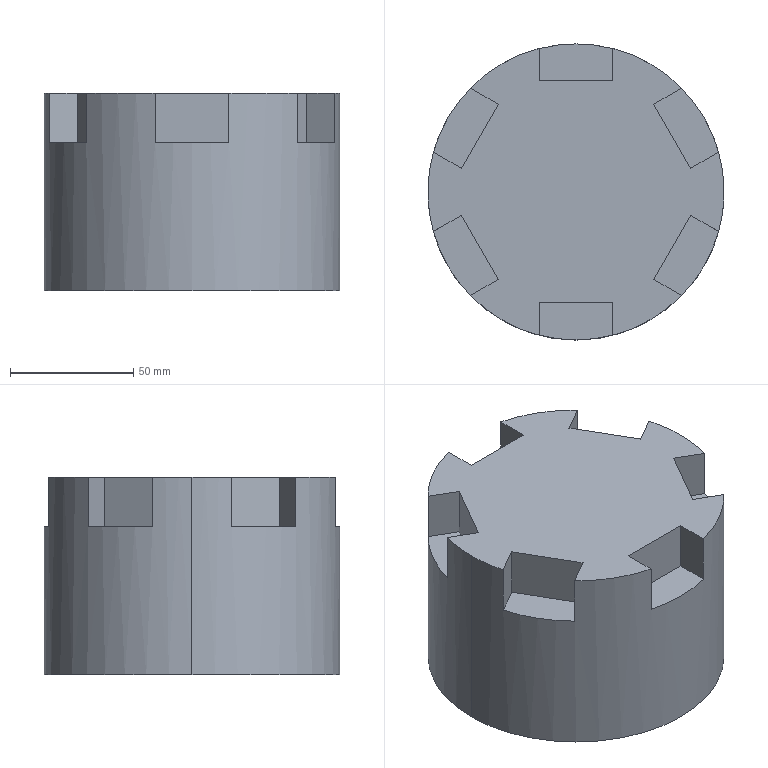Part | SolidWorks | features ICE 3, Extrusion 1 | 1 solid | 35 faces | box 120 x 120 x 80 mm | volume 586209 mm3 | plane 31 | cylinder 4 | commonest cylinder face diameters 75 x2 120 x2
STEP:
#1=CARTESIAN_POINT('',(60.,0.,80.));
#2=VERTEX_POINT('',#1);
#3=CARTESIAN_POINT('',(57.812,16.057,80.));
#4=VERTEX_POINT('',#3);
#5=CARTESIAN_POINT('',(0.,0.,80.));
#6=DIRECTION('',(0.,0.,1.));
#7=DIRECTION('',(1.,0.,0.));
#8=AXIS2_PLACEMENT_3D('',#5,#6,#7);
#9=CIRCLE('',#8,60.);
#10=EDGE_CURVE('',#2,#4,#9,.T.);
#11=ORIENTED_EDGE('',*,*,#10,.F.);
#12=CARTESIAN_POINT('',(60.,0.,0.));
#13=VERTEX_POINT('',#12);
#14=CARTESIAN_POINT('',(60.,0.,80.));
#15=DIRECTION('',(0.,0.,-1.));
#16=VECTOR('',#15,1000.);
#17=LINE('',#14,#16);
#18=EDGE_CURVE('',#2,#13,#17,.T.);
#19=ORIENTED_EDGE('',*,*,#18,.T.);
#20=CARTESIAN_POINT('',(-60.,0.,0.));
#21=VERTEX_POINT('',#20);
#22=CARTESIAN_POINT('',(0.,0.,0.));
#23=DIRECTION('',(0.,0.,1.));
#24=DIRECTION('',(1.,0.,0.));
#25=AXIS2_PLACEMENT_3D('',#22,#23,#24);
#26=CIRCLE('',#25,60.);
#27=EDGE_CURVE('',#13,#21,#26,.T.);
#28=ORIENTED_EDGE('',*,*,#27,.T.);
#29=CARTESIAN_POINT('',(-60.,0.,80.));
#30=VERTEX_POINT('',#29);
#31=CARTESIAN_POINT('',(-60.,0.,80.));
#32=DIRECTION('',(0.,0.,-1.));
#33=VECTOR('',#32,1000.);
#34=LINE('',#31,#33);
#35=EDGE_CURVE('',#30,#21,#34,.T.);
#36=ORIENTED_EDGE('',*,*,#35,.F.);
#37=CARTESIAN_POINT('',(-57.812,16.057,80.));
#38=VERTEX_POINT('',#37);
#39=CARTESIAN_POINT('',(0.,0.,80.));
#40=DIRECTION('',(0.,0.,1.));
#41=DIRECTION('',(1.,0.,0.));
#42=AXIS2_PLACEMENT_3D('',#39,#40,#41);
#43=CIRCLE('',#42,60.);
#44=EDGE_CURVE('',#38,#30,#43,.T.);
#45=ORIENTED_EDGE('',*,*,#44,.F.);
#46=CARTESIAN_POINT('',(-57.812,16.057,60.));
#47=VERTEX_POINT('',#46);
#48=CARTESIAN_POINT('',(-57.812,16.057,60.));
#49=DIRECTION('',(0.,0.,1.));
#50=VECTOR('',#49,1000.);
#51=LINE('',#48,#50);
#52=EDGE_CURVE('',#47,#38,#51,.T.);
#53=ORIENTED_EDGE('',*,*,#52,.F.);
#54=CARTESIAN_POINT('',(-42.812,42.038,60.));
#55=VERTEX_POINT('',#54);
#56=CARTESIAN_POINT('',(0.,0.,60.));
#57=DIRECTION('',(0.,0.,1.));
#58=DIRECTION('',(1.,0.,0.));
#59=AXIS2_PLACEMENT_3D('',#56,#57,#58);
#60=CIRCLE('',#59,60.);
#61=EDGE_CURVE('',#55,#47,#60,.T.);
#62=ORIENTED_EDGE('',*,*,#61,.F.);
#63=CARTESIAN_POINT('',(-42.812,42.038,80.));
#64=VERTEX_POINT('',#63);
#65=CARTESIAN_POINT('',(-42.812,42.038,60.));
#66=DIRECTION('',(0.,0.,1.));
#67=VECTOR('',#66,1000.);
#68=LINE('',#65,#67);
#69=EDGE_CURVE('',#55,#64,#68,.T.);
#70=ORIENTED_EDGE('',*,*,#69,.T.);
#71=CARTESIAN_POINT('',(-15.,58.095,80.));
#72=VERTEX_POINT('',#71);
#73=CARTESIAN_POINT('',(0.,0.,80.));
#74=DIRECTION('',(0.,0.,1.));
#75=DIRECTION('',(1.,0.,0.));
#76=AXIS2_PLACEMENT_3D('',#73,#74,#75);
#77=CIRCLE('',#76,60.);
#78=EDGE_CURVE('',#72,#64,#77,.T.);
#79=ORIENTED_EDGE('',*,*,#78,.F.);
#80=CARTESIAN_POINT('',(-15.,58.095,60.));
#81=VERTEX_POINT('',#80);
#82=CARTESIAN_POINT('',(-15.,58.095,60.));
#83=DIRECTION('',(0.,0.,1.));
#84=VECTOR('',#83,1000.);
#85=LINE('',#82,#84);
#86=EDGE_CURVE('',#81,#72,#85,.T.);
#87=ORIENTED_EDGE('',*,*,#86,.F.);
#88=CARTESIAN_POINT('',(15.,58.095,60.));
#89=VERTEX_POINT('',#88);
#90=CARTESIAN_POINT('',(0.,0.,60.));
#91=DIRECTION('',(0.,0.,1.));
#92=DIRECTION('',(1.,0.,0.));
#93=AXIS2_PLACEMENT_3D('',#90,#91,#92);
#94=CIRCLE('',#93,60.);
#95=EDGE_CURVE('',#89,#81,#94,.T.);
#96=ORIENTED_EDGE('',*,*,#95,.F.);
#97=CARTESIAN_POINT('',(15.,58.095,80.));
#98=VERTEX_POINT('',#97);
#99=CARTESIAN_POINT('',(15.,58.095,60.));
#100=DIRECTION('',(0.,0.,1.));
#101=VECTOR('',#100,1000.);
#102=LINE('',#99,#101);
#103=EDGE_CURVE('',#89,#98,#102,.T.);
#104=ORIENTED_EDGE('',*,*,#103,.T.);
#105=CARTESIAN_POINT('',(42.812,42.038,80.));
#106=VERTEX_POINT('',#105);
#107=CARTESIAN_POINT('',(0.,0.,80.));
#108=DIRECTION('',(0.,0.,1.));
#109=DIRECTION('',(1.,0.,0.));
#110=AXIS2_PLACEMENT_3D('',#107,#108,#109);
#111=CIRCLE('',#110,60.);
#112=EDGE_CURVE('',#106,#98,#111,.T.);
#113=ORIENTED_EDGE('',*,*,#112,.F.);
#114=CARTESIAN_POINT('',(42.812,42.038,60.));
#115=VERTEX_POINT('',#114);
#116=CARTESIAN_POINT('',(42.812,42.038,60.));
#117=DIRECTION('',(0.,0.,1.));
#118=VECTOR('',#117,1000.);
#119=LINE('',#116,#118);
#120=EDGE_CURVE('',#115,#106,#119,.T.);
#121=ORIENTED_EDGE('',*,*,#120,.F.);
#122=CARTESIAN_POINT('',(57.812,16.057,60.));
#123=VERTEX_POINT('',#122);
#124=CARTESIAN_POINT('',(0.,0.,60.));
#125=DIRECTION('',(0.,0.,1.));
#126=DIRECTION('',(1.,0.,0.));
#127=AXIS2_PLACEMENT_3D('',#124,#125,#126);
#128=CIRCLE('',#127,60.);
#129=EDGE_CURVE('',#123,#115,#128,.T.);
#130=ORIENTED_EDGE('',*,*,#129,.F.);
#131=CARTESIAN_POINT('',(57.812,16.057,60.));
#132=DIRECTION('',(0.,0.,1.));
#133=VECTOR('',#132,1000.);
#134=LINE('',#131,#133);
#135=EDGE_CURVE('',#123,#4,#134,.T.);
#136=ORIENTED_EDGE('',*,*,#135,.T.);
#137=EDGE_LOOP('',(#11,#19,#28,#36,#45,#53,#62,#70,#79,#87,#96,#104,#113,#121,#130,#136));
#138=FACE_OUTER_BOUND('',#137,.T.);
#139=CARTESIAN_POINT('',(0.,0.,80.));
#140=DIRECTION('',(0.,0.,-1.));
#141=DIRECTION('',(-1.,0.,0.));
#142=AXIS2_PLACEMENT_3D('',#139,#140,#141);
#143=CYLINDRICAL_SURFACE('',#142,60.);
#144=ADVANCED_FACE('',(#138),#143,.T.);
#145=CARTESIAN_POINT('',(-37.5,0.,60.));
#146=VERTEX_POINT('',#145);
#147=CARTESIAN_POINT('',(37.5,0.,60.));
#148=VERTEX_POINT('',#147);
#149=CARTESIAN_POINT('',(0.,0.,60.));
#150=DIRECTION('',(0.,0.,1.));
#151=DIRECTION('',(1.,0.,0.));
#152=AXIS2_PLACEMENT_3D('',#149,#150,#151);
#153=CIRCLE('',#152,37.5);
#154=EDGE_CURVE('',#146,#148,#153,.T.);
#155=ORIENTED_EDGE('',*,*,#154,.T.);
#156=CARTESIAN_POINT('',(37.5,0.,0.));
#157=VERTEX_POINT('',#156);
#158=CARTESIAN_POINT('',(37.5,0.,60.));
#159=DIRECTION('',(0.,0.,-1.));
#160=VECTOR('',#159,1000.);
#161=LINE('',#158,#160);
#162=EDGE_CURVE('',#148,#157,#161,.T.);
#163=ORIENTED_EDGE('',*,*,#162,.T.);
#164=CARTESIAN_POINT('',(-37.5,0.,0.));
#165=VERTEX_POINT('',#164);
#166=CARTESIAN_POINT('',(0.,0.,0.));
#167=DIRECTION('',(0.,0.,1.));
#168=DIRECTION('',(1.,0.,0.));
#169=AXIS2_PLACEMENT_3D('',#166,#167,#168);
#170=CIRCLE('',#169,37.5);
#171=EDGE_CURVE('',#165,#157,#170,.T.);
#172=ORIENTED_EDGE('',*,*,#171,.F.);
#173=CARTESIAN_POINT('',(-37.5,0.,60.));
#174=DIRECTION('',(0.,0.,-1.));
#175=VECTOR('',#174,1000.);
#176=LINE('',#173,#175);
#177=EDGE_CURVE('',#146,#165,#176,.T.);
#178=ORIENTED_EDGE('',*,*,#177,.F.);
#179=EDGE_LOOP('',(#155,#163,#172,#178));
#180=FACE_OUTER_BOUND('',#179,.T.);
#181=CARTESIAN_POINT('',(0.,0.,60.));
#182=DIRECTION('',(0.,0.,-1.));
#183=DIRECTION('',(-1.,0.,0.));
#184=AXIS2_PLACEMENT_3D('',#181,#182,#183);
#185=CYLINDRICAL_SURFACE('',#184,37.5);
#186=ADVANCED_FACE('',(#180),#185,.F.);
#187=CARTESIAN_POINT('',(0.,0.,0.));
#188=DIRECTION('',(0.,0.,1.));
#189=DIRECTION('',(1.,0.,0.));
#190=AXIS2_PLACEMENT_3D('',#187,#188,#189);
#191=CIRCLE('',#190,60.);
#192=EDGE_CURVE('',#21,#13,#191,.T.);
#193=ORIENTED_EDGE('',*,*,#192,.F.);
#194=ORIENTED_EDGE('',*,*,#27,.F.);
#195=EDGE_LOOP('',(#193,#194));
#196=FACE_OUTER_BOUND('',#195,.T.);
#197=CARTESIAN_POINT('',(-10.,40.,0.));
#198=VERTEX_POINT('',#197);
#199=CARTESIAN_POINT('',(-10.,36.142,0.));
#200=VERTEX_POINT('',#199);
#201=CARTESIAN_POINT('',(-10.,40.,0.));
#202=DIRECTION('',(0.,-1.,0.));
#203=VECTOR('',#202,1000.);
#204=LINE('',#201,#203);
#205=EDGE_CURVE('',#198,#200,#204,.T.);
#206=ORIENTED_EDGE('',*,*,#205,.T.);
#207=CARTESIAN_POINT('',(0.,0.,0.));
#208=DIRECTION('',(0.,0.,1.));
#209=DIRECTION('',(1.,0.,0.));
#210=AXIS2_PLACEMENT_3D('',#207,#208,#209);
#211=CIRCLE('',#210,37.5);
#212=EDGE_CURVE('',#200,#165,#211,.T.);
#213=ORIENTED_EDGE('',*,*,#212,.T.);
#214=ORIENTED_EDGE('',*,*,#171,.T.);
#215=CARTESIAN_POINT('',(10.,36.142,0.));
#216=VERTEX_POINT('',#215);
#217=CARTESIAN_POINT('',(0.,0.,0.));
#218=DIRECTION('',(0.,0.,1.));
#219=DIRECTION('',(1.,0.,0.));
#220=AXIS2_PLACEMENT_3D('',#217,#218,#219);
#221=CIRCLE('',#220,37.5);
#222=EDGE_CURVE('',#157,#216,#221,.T.);
#223=ORIENTED_EDGE('',*,*,#222,.T.);
#224=CARTESIAN_POINT('',(10.,40.,0.));
#225=VERTEX_POINT('',#224);
#226=CARTESIAN_POINT('',(10.,40.,0.));
#227=DIRECTION('',(0.,-1.,0.));
#228=VECTOR('',#227,1000.);
#229=LINE('',#226,#228);
#230=EDGE_CURVE('',#225,#216,#229,.T.);
#231=ORIENTED_EDGE('',*,*,#230,.F.);
#232=CARTESIAN_POINT('',(10.,40.,0.));
#233=DIRECTION('',(-1.,0.,0.));
#234=VECTOR('',#233,1000.);
#235=LINE('',#232,#234);
#236=EDGE_CURVE('',#225,#198,#235,.T.);
#237=ORIENTED_EDGE('',*,*,#236,.T.);
#238=EDGE_LOOP('',(#206,#213,#214,#223,#231,#237));
#239=FACE_BOUND('',#238,.T.);
#240=CARTESIAN_POINT('',(0.,0.,0.));
#241=DIRECTION('',(0.,0.,1.));
#242=DIRECTION('',(1.,0.,0.));
#243=AXIS2_PLACEMENT_3D('',#240,#241,#242);
#244=PLANE('',#243);
#245=ADVANCED_FACE('',(#196,#239),#244,.F.);
#246=ORIENTED_EDGE('',*,*,#162,.F.);
#247=CARTESIAN_POINT('',(0.,0.,60.));
#248=DIRECTION('',(0.,0.,1.));
#249=DIRECTION('',(1.,0.,0.));
#250=AXIS2_PLACEMENT_3D('',#247,#248,#249);
#251=CIRCLE('',#250,37.5);
#252=EDGE_CURVE('',#148,#146,#251,.T.);
#253=ORIENTED_EDGE('',*,*,#252,.T.);
#254=ORIENTED_EDGE('',*,*,#177,.T.);
#255=ORIENTED_EDGE('',*,*,#212,.F.);
#256=CARTESIAN_POINT('',(-10.,36.142,30.));
#257=VERTEX_POINT('',#256);
#258=CARTESIAN_POINT('',(-10.,36.142,60.));
#259=DIRECTION('',(0.,0.,1.));
#260=VECTOR('',#259,1000.);
#261=LINE('',#258,#260);
#262=EDGE_CURVE('',#200,#257,#261,.T.);
#263=ORIENTED_EDGE('',*,*,#262,.T.);
#264=CARTESIAN_POINT('',(10.,36.142,30.));
#265=VERTEX_POINT('',#264);
#266=CARTESIAN_POINT('',(0.,0.,30.));
#267=DIRECTION('',(0.,0.,1.));
#268=DIRECTION('',(1.,0.,0.));
#269=AXIS2_PLACEMENT_3D('',#266,#267,#268);
#270=CIRCLE('',#269,37.5);
#271=EDGE_CURVE('',#265,#257,#270,.T.);
#272=ORIENTED_EDGE('',*,*,#271,.F.);
#273=CARTESIAN_POINT('',(10.,36.142,60.));
#274=DIRECTION('',(0.,0.,1.));
#275=VECTOR('',#274,1000.);
#276=LINE('',#273,#275);
#277=EDGE_CURVE('',#216,#265,#276,.T.);
#278=ORIENTED_EDGE('',*,*,#277,.F.);
#279=ORIENTED_EDGE('',*,*,#222,.F.);
#280=EDGE_LOOP('',(#246,#253,#254,#255,#263,#272,#278,#279));
#281=FACE_OUTER_BOUND('',#280,.T.);
#282=CARTESIAN_POINT('',(0.,0.,60.));
#283=DIRECTION('',(0.,0.,-1.));
#284=DIRECTION('',(-1.,0.,0.));
#285=AXIS2_PLACEMENT_3D('',#282,#283,#284);
#286=CYLINDRICAL_SURFACE('',#285,37.5);
#287=ADVANCED_FACE('',(#281),#286,.F.);
#288=ORIENTED_EDGE('',*,*,#18,.F.);
#289=CARTESIAN_POINT('',(57.812,-16.057,80.));
#290=VERTEX_POINT('',#289);
#291=CARTESIAN_POINT('',(0.,0.,80.));
#292=DIRECTION('',(0.,0.,1.));
#293=DIRECTION('',(1.,0.,0.));
#294=AXIS2_PLACEMENT_3D('',#291,#292,#293);
#295=CIRCLE('',#294,60.);
#296=EDGE_CURVE('',#290,#2,#295,.T.);
#297=ORIENTED_EDGE('',*,*,#296,.F.);
#298=CARTESIAN_POINT('',(57.812,-16.057,60.));
#299=VERTEX_POINT('',#298);
#300=CARTESIAN_POINT('',(57.812,-16.057,60.));
#301=DIRECTION('',(0.,0.,1.));
#302=VECTOR('',#301,1000.);
#303=LINE('',#300,#302);
#304=EDGE_CURVE('',#299,#290,#303,.T.);
#305=ORIENTED_EDGE('',*,*,#304,.F.);
#306=CARTESIAN_POINT('',(42.812,-42.038,60.));
#307=VERTEX_POINT('',#306);
#308=CARTESIAN_POINT('',(0.,0.,60.));
#309=DIRECTION('',(0.,0.,1.));
#310=DIRECTION('',(1.,0.,0.));
#311=AXIS2_PLACEMENT_3D('',#308,#309,#310);
#312=CIRCLE('',#311,60.);
#313=EDGE_CURVE('',#307,#299,#312,.T.);
#314=ORIENTED_EDGE('',*,*,#313,.F.);
#315=CARTESIAN_POINT('',(42.812,-42.038,80.));
#316=VERTEX_POINT('',#315);
#317=CARTESIAN_POINT('',(42.812,-42.038,60.));
#318=DIRECTION('',(0.,0.,1.));
#319=VECTOR('',#318,1000.);
#320=LINE('',#317,#319);
#321=EDGE_CURVE('',#307,#316,#320,.T.);
#322=ORIENTED_EDGE('',*,*,#321,.T.);
#323=CARTESIAN_POINT('',(15.,-58.095,80.));
#324=VERTEX_POINT('',#323);
#325=CARTESIAN_POINT('',(0.,0.,80.));
#326=DIRECTION('',(0.,0.,1.));
#327=DIRECTION('',(1.,0.,0.));
#328=AXIS2_PLACEMENT_3D('',#325,#326,#327);
#329=CIRCLE('',#328,60.);
#330=EDGE_CURVE('',#324,#316,#329,.T.);
#331=ORIENTED_EDGE('',*,*,#330,.F.);
#332=CARTESIAN_POINT('',(15.,-58.095,60.));
#333=VERTEX_POINT('',#332);
#334=CARTESIAN_POINT('',(15.,-58.095,60.));
#335=DIRECTION('',(0.,0.,1.));
#336=VECTOR('',#335,1000.);
#337=LINE('',#334,#336);
#338=EDGE_CURVE('',#333,#324,#337,.T.);
#339=ORIENTED_EDGE('',*,*,#338,.F.);
#340=CARTESIAN_POINT('',(-15.,-58.095,60.));
#341=VERTEX_POINT('',#340);
#342=CARTESIAN_POINT('',(0.,0.,60.));
#343=DIRECTION('',(0.,0.,1.));
#344=DIRECTION('',(1.,0.,0.));
#345=AXIS2_PLACEMENT_3D('',#342,#343,#344);
#346=CIRCLE('',#345,60.);
#347=EDGE_CURVE('',#341,#333,#346,.T.);
#348=ORIENTED_EDGE('',*,*,#347,.F.);
#349=CARTESIAN_POINT('',(-15.,-58.095,80.));
#350=VERTEX_POINT('',#349);
#351=CARTESIAN_POINT('',(-15.,-58.095,60.));
#352=DIRECTION('',(0.,0.,1.));
#353=VECTOR('',#352,1000.);
#354=LINE('',#351,#353);
#355=EDGE_CURVE('',#341,#350,#354,.T.);
#356=ORIENTED_EDGE('',*,*,#355,.T.);
#357=CARTESIAN_POINT('',(-42.812,-42.038,80.));
#358=VERTEX_POINT('',#357);
#359=CARTESIAN_POINT('',(0.,0.,80.));
#360=DIRECTION('',(0.,0.,1.));
#361=DIRECTION('',(1.,0.,0.));
#362=AXIS2_PLACEMENT_3D('',#359,#360,#361);
#363=CIRCLE('',#362,60.);
#364=EDGE_CURVE('',#358,#350,#363,.T.);
#365=ORIENTED_EDGE('',*,*,#364,.F.);
#366=CARTESIAN_POINT('',(-42.812,-42.038,60.));
#367=VERTEX_POINT('',#366);
#368=CARTESIAN_POINT('',(-42.812,-42.038,60.));
#369=DIRECTION('',(0.,0.,1.));
#370=VECTOR('',#369,1000.);
#371=LINE('',#368,#370);
#372=EDGE_CURVE('',#367,#358,#371,.T.);
#373=ORIENTED_EDGE('',*,*,#372,.F.);
#374=CARTESIAN_POINT('',(-57.812,-16.057,60.));
#375=VERTEX_POINT('',#374);
#376=CARTESIAN_POINT('',(0.,0.,60.));
#377=DIRECTION('',(0.,0.,1.));
#378=DIRECTION('',(1.,0.,0.));
#379=AXIS2_PLACEMENT_3D('',#376,#377,#378);
#380=CIRCLE('',#379,60.);
#381=EDGE_CURVE('',#375,#367,#380,.T.);
#382=ORIENTED_EDGE('',*,*,#381,.F.);
#383=CARTESIAN_POINT('',(-57.812,-16.057,80.));
#384=VERTEX_POINT('',#383);
#385=CARTESIAN_POINT('',(-57.812,-16.057,60.));
#386=DIRECTION('',(0.,0.,1.));
#387=VECTOR('',#386,1000.);
#388=LINE('',#385,#387);
#389=EDGE_CURVE('',#375,#384,#388,.T.);
#390=ORIENTED_EDGE('',*,*,#389,.T.);
#391=CARTESIAN_POINT('',(0.,0.,80.));
#392=DIRECTION('',(0.,0.,1.));
#393=DIRECTION('',(1.,0.,0.));
#394=AXIS2_PLACEMENT_3D('',#391,#392,#393);
#395=CIRCLE('',#394,60.);
#396=EDGE_CURVE('',#30,#384,#395,.T.);
#397=ORIENTED_EDGE('',*,*,#396,.F.);
#398=ORIENTED_EDGE('',*,*,#35,.T.);
#399=ORIENTED_EDGE('',*,*,#192,.T.);
#400=EDGE_LOOP('',(#288,#297,#305,#314,#322,#331,#339,#348,#356,#365,#373,#382,#390,#397,#398,#399));
#401=FACE_OUTER_BOUND('',#400,.T.);
#402=CARTESIAN_POINT('',(0.,0.,80.));
#403=DIRECTION('',(0.,0.,-1.));
#404=DIRECTION('',(-1.,0.,0.));
#405=AXIS2_PLACEMENT_3D('',#402,#403,#404);
#406=CYLINDRICAL_SURFACE('',#405,60.);
#407=ADVANCED_FACE('',(#401),#406,.T.);
#408=CARTESIAN_POINT('',(15.,45.,80.));
#409=VERTEX_POINT('',#408);
#410=CARTESIAN_POINT('',(15.,58.095,80.));
#411=DIRECTION('',(0.,1.,0.));
#412=VECTOR('',#411,1000.);
#413=LINE('',#410,#412);
#414=EDGE_CURVE('',#409,#98,#413,.T.);
#415=ORIENTED_EDGE('',*,*,#414,.F.);
#416=CARTESIAN_POINT('',(-15.,45.,80.));
#417=VERTEX_POINT('',#416);
#418=CARTESIAN_POINT('',(-15.,45.,80.));
#419=DIRECTION('',(1.,0.,0.));
#420=VECTOR('',#419,1000.);
#421=LINE('',#418,#420);
#422=EDGE_CURVE('',#417,#409,#421,.T.);
#423=ORIENTED_EDGE('',*,*,#422,.F.);
#424=CARTESIAN_POINT('',(-15.,58.095,80.));
#425=DIRECTION('',(0.,-1.,0.));
#426=VECTOR('',#425,1000.);
#427=LINE('',#424,#426);
#428=EDGE_CURVE('',#72,#417,#427,.T.);
#429=ORIENTED_EDGE('',*,*,#428,.F.);
#430=ORIENTED_EDGE('',*,*,#78,.T.);
#431=CARTESIAN_POINT('',(-31.471,35.49,80.));
#432=VERTEX_POINT('',#431);
#433=CARTESIAN_POINT('',(-42.812,42.038,80.));
#434=DIRECTION('',(-0.866,0.5,0.));
#435=VECTOR('',#434,1000.);
#436=LINE('',#433,#435);
#437=EDGE_CURVE('',#432,#64,#436,.T.);
#438=ORIENTED_EDGE('',*,*,#437,.F.);
#439=CARTESIAN_POINT('',(-46.471,9.51,80.));
#440=VERTEX_POINT('',#439);
#441=CARTESIAN_POINT('',(-46.471,9.51,80.));
#442=DIRECTION('',(0.5,0.866,0.));
#443=VECTOR('',#442,1000.);
#444=LINE('',#441,#443);
#445=EDGE_CURVE('',#440,#432,#444,.T.);
#446=ORIENTED_EDGE('',*,*,#445,.F.);
#447=CARTESIAN_POINT('',(-57.812,16.057,80.));
#448=DIRECTION('',(0.866,-0.5,0.));
#449=VECTOR('',#448,1000.);
#450=LINE('',#447,#449);
#451=EDGE_CURVE('',#38,#440,#450,.T.);
#452=ORIENTED_EDGE('',*,*,#451,.F.);
#453=ORIENTED_EDGE('',*,*,#44,.T.);
#454=ORIENTED_EDGE('',*,*,#396,.T.);
#455=CARTESIAN_POINT('',(-46.471,-9.51,80.));
#456=VERTEX_POINT('',#455);
#457=CARTESIAN_POINT('',(-57.812,-16.057,80.));
#458=DIRECTION('',(-0.866,-0.5,0.));
#459=VECTOR('',#458,1000.);
#460=LINE('',#457,#459);
#461=EDGE_CURVE('',#456,#384,#460,.T.);
#462=ORIENTED_EDGE('',*,*,#461,.F.);
#463=CARTESIAN_POINT('',(-31.471,-35.49,80.));
#464=VERTEX_POINT('',#463);
#465=CARTESIAN_POINT('',(-31.471,-35.49,80.));
#466=DIRECTION('',(-0.5,0.866,0.));
#467=VECTOR('',#466,1000.);
#468=LINE('',#465,#467);
#469=EDGE_CURVE('',#464,#456,#468,.T.);
#470=ORIENTED_EDGE('',*,*,#469,.F.);
#471=CARTESIAN_POINT('',(-42.812,-42.038,80.));
#472=DIRECTION('',(0.866,0.5,0.));
#473=VECTOR('',#472,1000.);
#474=LINE('',#471,#473);
#475=EDGE_CURVE('',#358,#464,#474,.T.);
#476=ORIENTED_EDGE('',*,*,#475,.F.);
#477=ORIENTED_EDGE('',*,*,#364,.T.);
#478=CARTESIAN_POINT('',(-15.,-45.,80.));
#479=VERTEX_POINT('',#478);
#480=CARTESIAN_POINT('',(-15.,-58.095,80.));
#481=DIRECTION('',(0.,-1.,0.));
#482=VECTOR('',#481,1000.);
#483=LINE('',#480,#482);
#484=EDGE_CURVE('',#479,#350,#483,.T.);
#485=ORIENTED_EDGE('',*,*,#484,.F.);
#486=CARTESIAN_POINT('',(15.,-45.,80.));
#487=VERTEX_POINT('',#486);
#488=CARTESIAN_POINT('',(15.,-45.,80.));
#489=DIRECTION('',(-1.,0.,0.));
#490=VECTOR('',#489,1000.);
#491=LINE('',#488,#490);
#492=EDGE_CURVE('',#487,#479,#491,.T.);
#493=ORIENTED_EDGE('',*,*,#492,.F.);
#494=CARTESIAN_POINT('',(15.,-58.095,80.));
#495=DIRECTION('',(0.,1.,0.));
#496=VECTOR('',#495,1000.);
#497=LINE('',#494,#496);
#498=EDGE_CURVE('',#324,#487,#497,.T.);
#499=ORIENTED_EDGE('',*,*,#498,.F.);
#500=ORIENTED_EDGE('',*,*,#330,.T.);
#501=CARTESIAN_POINT('',(31.471,-35.49,80.));
#502=VERTEX_POINT('',#501);
#503=CARTESIAN_POINT('',(42.812,-42.038,80.));
#504=DIRECTION('',(0.866,-0.5,0.));
#505=VECTOR('',#504,1000.);
#506=LINE('',#503,#505);
#507=EDGE_CURVE('',#502,#316,#506,.T.);
#508=ORIENTED_EDGE('',*,*,#507,.F.);
#509=CARTESIAN_POINT('',(46.471,-9.51,80.));
#510=VERTEX_POINT('',#509);
#511=CARTESIAN_POINT('',(46.471,-9.51,80.));
#512=DIRECTION('',(-0.5,-0.866,0.));
#513=VECTOR('',#512,1000.);
#514=LINE('',#511,#513);
#515=EDGE_CURVE('',#510,#502,#514,.T.);
#516=ORIENTED_EDGE('',*,*,#515,.F.);
#517=CARTESIAN_POINT('',(57.812,-16.057,80.));
#518=DIRECTION('',(-0.866,0.5,0.));
#519=VECTOR('',#518,1000.);
#520=LINE('',#517,#519);
#521=EDGE_CURVE('',#290,#510,#520,.T.);
#522=ORIENTED_EDGE('',*,*,#521,.F.);
#523=ORIENTED_EDGE('',*,*,#296,.T.);
#524=ORIENTED_EDGE('',*,*,#10,.T.);
#525=CARTESIAN_POINT('',(46.471,9.51,80.));
#526=VERTEX_POINT('',#525);
#527=CARTESIAN_POINT('',(57.812,16.057,80.));
#528=DIRECTION('',(0.866,0.5,0.));
#529=VECTOR('',#528,1000.);
#530=LINE('',#527,#529);
#531=EDGE_CURVE('',#526,#4,#530,.T.);
#532=ORIENTED_EDGE('',*,*,#531,.F.);
#533=CARTESIAN_POINT('',(31.471,35.49,80.));
#534=VERTEX_POINT('',#533);
#535=CARTESIAN_POINT('',(31.471,35.49,80.));
#536=DIRECTION('',(0.5,-0.866,0.));
#537=VECTOR('',#536,1000.);
#538=LINE('',#535,#537);
#539=EDGE_CURVE('',#534,#526,#538,.T.);
#540=ORIENTED_EDGE('',*,*,#539,.F.);
#541=CARTESIAN_POINT('',(42.812,42.038,80.));
#542=DIRECTION('',(-0.866,-0.5,0.));
#543=VECTOR('',#542,1000.);
#544=LINE('',#541,#543);
#545=EDGE_CURVE('',#106,#534,#544,.T.);
#546=ORIENTED_EDGE('',*,*,#545,.F.);
#547=ORIENTED_EDGE('',*,*,#112,.T.);
#548=EDGE_LOOP('',(#415,#423,#429,#430,#438,#446,#452,#453,#454,#462,#470,#476,#477,#485,#493,#499,#500,#508,#516,#522,#523,#524,#532,#540,#546,#547));
#549=FACE_OUTER_BOUND('',#548,.T.);
#550=CARTESIAN_POINT('',(0.,0.,80.));
#551=DIRECTION('',(0.,0.,1.));
#552=DIRECTION('',(1.,0.,0.));
#553=AXIS2_PLACEMENT_3D('',#550,#551,#552);
#554=PLANE('',#553);
#555=ADVANCED_FACE('',(#549),#554,.T.);
#556=ORIENTED_EDGE('',*,*,#154,.F.);
#557=ORIENTED_EDGE('',*,*,#252,.F.);
#558=EDGE_LOOP('',(#556,#557));
#559=FACE_OUTER_BOUND('',#558,.T.);
#560=CARTESIAN_POINT('',(0.,0.,60.));
#561=DIRECTION('',(0.,0.,1.));
#562=DIRECTION('',(1.,0.,0.));
#563=AXIS2_PLACEMENT_3D('',#560,#561,#562);
#564=PLANE('',#563);
#565=ADVANCED_FACE('',(#559),#564,.F.);
#566=ORIENTED_EDGE('',*,*,#539,.T.);
#567=CARTESIAN_POINT('',(46.471,9.51,60.));
#568=VERTEX_POINT('',#567);
#569=CARTESIAN_POINT('',(46.471,9.51,60.));
#570=DIRECTION('',(0.,0.,1.));
#571=VECTOR('',#570,1000.);
#572=LINE('',#569,#571);
#573=EDGE_CURVE('',#568,#526,#572,.T.);
#574=ORIENTED_EDGE('',*,*,#573,.F.);
#575=CARTESIAN_POINT('',(31.471,35.49,60.));
#576=VERTEX_POINT('',#575);
#577=CARTESIAN_POINT('',(31.471,35.49,60.));
#578=DIRECTION('',(0.5,-0.866,0.));
#579=VECTOR('',#578,1000.);
#580=LINE('',#577,#579);
#581=EDGE_CURVE('',#576,#568,#580,.T.);
#582=ORIENTED_EDGE('',*,*,#581,.F.);
#583=CARTESIAN_POINT('',(31.471,35.49,60.));
#584=DIRECTION('',(0.,0.,1.));
#585=VECTOR('',#584,1000.);
#586=LINE('',#583,#585);
#587=EDGE_CURVE('',#576,#534,#586,.T.);
#588=ORIENTED_EDGE('',*,*,#587,.T.);
#589=EDGE_LOOP('',(#566,#574,#582,#588));
#590=FACE_OUTER_BOUND('',#589,.T.);
#591=CARTESIAN_POINT('',(31.471,35.49,60.));
#592=DIRECTION('',(-0.866,-0.5,0.));
#593=DIRECTION('',(0.5,-0.866,0.));
#594=AXIS2_PLACEMENT_3D('',#591,#592,#593);
#595=PLANE('',#594);
#596=ADVANCED_FACE('',(#590),#595,.F.);
#597=ORIENTED_EDGE('',*,*,#545,.T.);
#598=ORIENTED_EDGE('',*,*,#587,.F.);
#599=CARTESIAN_POINT('',(42.812,42.038,60.));
#600=DIRECTION('',(-0.866,-0.5,0.));
#601=VECTOR('',#600,1000.);
#602=LINE('',#599,#601);
#603=EDGE_CURVE('',#115,#576,#602,.T.);
#604=ORIENTED_EDGE('',*,*,#603,.F.);
#605=ORIENTED_EDGE('',*,*,#120,.T.);
#606=EDGE_LOOP('',(#597,#598,#604,#605));
#607=FACE_OUTER_BOUND('',#606,.T.);
#608=CARTESIAN_POINT('',(42.812,42.038,60.));
#609=DIRECTION('',(-0.5,0.866,0.));
#610=DIRECTION('',(-0.866,-0.5,0.));
#611=AXIS2_PLACEMENT_3D('',#608,#609,#610);
#612=PLANE('',#611);
#613=ADVANCED_FACE('',(#607),#612,.F.);
#614=ORIENTED_EDGE('',*,*,#531,.T.);
#615=ORIENTED_EDGE('',*,*,#135,.F.);
#616=CARTESIAN_POINT('',(57.812,16.057,60.));
#617=DIRECTION('',(0.866,0.5,0.));
#618=VECTOR('',#617,1000.);
#619=LINE('',#616,#618);
#620=EDGE_CURVE('',#568,#123,#619,.T.);
#621=ORIENTED_EDGE('',*,*,#620,.F.);
#622=ORIENTED_EDGE('',*,*,#573,.T.);
#623=EDGE_LOOP('',(#614,#615,#621,#622));
#624=FACE_OUTER_BOUND('',#623,.T.);
#625=CARTESIAN_POINT('',(57.812,16.057,60.));
#626=DIRECTION('',(0.5,-0.866,0.));
#627=DIRECTION('',(0.866,0.5,0.));
#628=AXIS2_PLACEMENT_3D('',#625,#626,#627);
#629=PLANE('',#628);
#630=ADVANCED_FACE('',(#624),#629,.F.);
#631=ORIENTED_EDGE('',*,*,#581,.T.);
#632=ORIENTED_EDGE('',*,*,#620,.T.);
#633=ORIENTED_EDGE('',*,*,#129,.T.);
#634=ORIENTED_EDGE('',*,*,#603,.T.);
#635=EDGE_LOOP('',(#631,#632,#633,#634));
#636=FACE_OUTER_BOUND('',#635,.T.);
#637=CARTESIAN_POINT('',(0.,0.,60.));
#638=DIRECTION('',(0.,0.,1.));
#639=DIRECTION('',(1.,0.,0.));
#640=AXIS2_PLACEMENT_3D('',#637,#638,#639);
#641=PLANE('',#640);
#642=ADVANCED_FACE('',(#636),#641,.T.);
#643=ORIENTED_EDGE('',*,*,#515,.T.);
#644=CARTESIAN_POINT('',(31.471,-35.49,60.));
#645=VERTEX_POINT('',#644);
#646=CARTESIAN_POINT('',(31.471,-35.49,60.));
#647=DIRECTION('',(0.,0.,1.));
#648=VECTOR('',#647,1000.);
#649=LINE('',#646,#648);
#650=EDGE_CURVE('',#645,#502,#649,.T.);
#651=ORIENTED_EDGE('',*,*,#650,.F.);
#652=CARTESIAN_POINT('',(46.471,-9.51,60.));
#653=VERTEX_POINT('',#652);
#654=CARTESIAN_POINT('',(46.471,-9.51,60.));
#655=DIRECTION('',(-0.5,-0.866,0.));
#656=VECTOR('',#655,1000.);
#657=LINE('',#654,#656);
#658=EDGE_CURVE('',#653,#645,#657,.T.);
#659=ORIENTED_EDGE('',*,*,#658,.F.);
#660=CARTESIAN_POINT('',(46.471,-9.51,60.));
#661=DIRECTION('',(0.,0.,1.));
#662=VECTOR('',#661,1000.);
#663=LINE('',#660,#662);
#664=EDGE_CURVE('',#653,#510,#663,.T.);
#665=ORIENTED_EDGE('',*,*,#664,.T.);
#666=EDGE_LOOP('',(#643,#651,#659,#665));
#667=FACE_OUTER_BOUND('',#666,.T.);
#668=CARTESIAN_POINT('',(46.471,-9.51,60.));
#669=DIRECTION('',(-0.866,0.5,0.));
#670=DIRECTION('',(-0.5,-0.866,0.));
#671=AXIS2_PLACEMENT_3D('',#668,#669,#670);
#672=PLANE('',#671);
#673=ADVANCED_FACE('',(#667),#672,.F.);
#674=ORIENTED_EDGE('',*,*,#521,.T.);
#675=ORIENTED_EDGE('',*,*,#664,.F.);
#676=CARTESIAN_POINT('',(57.812,-16.057,60.));
#677=DIRECTION('',(-0.866,0.5,0.));
#678=VECTOR('',#677,1000.);
#679=LINE('',#676,#678);
#680=EDGE_CURVE('',#299,#653,#679,.T.);
#681=ORIENTED_EDGE('',*,*,#680,.F.);
#682=ORIENTED_EDGE('',*,*,#304,.T.);
#683=EDGE_LOOP('',(#674,#675,#681,#682));
#684=FACE_OUTER_BOUND('',#683,.T.);
#685=CARTESIAN_POINT('',(57.812,-16.057,60.));
#686=DIRECTION('',(0.5,0.866,0.));
#687=DIRECTION('',(-0.866,0.5,0.));
#688=AXIS2_PLACEMENT_3D('',#685,#686,#687);
#689=PLANE('',#688);
#690=ADVANCED_FACE('',(#684),#689,.F.);
#691=ORIENTED_EDGE('',*,*,#507,.T.);
#692=ORIENTED_EDGE('',*,*,#321,.F.);
#693=CARTESIAN_POINT('',(42.812,-42.038,60.));
#694=DIRECTION('',(0.866,-0.5,0.));
#695=VECTOR('',#694,1000.);
#696=LINE('',#693,#695);
#697=EDGE_CURVE('',#645,#307,#696,.T.);
#698=ORIENTED_EDGE('',*,*,#697,.F.);
#699=ORIENTED_EDGE('',*,*,#650,.T.);
#700=EDGE_LOOP('',(#691,#692,#698,#699));
#701=FACE_OUTER_BOUND('',#700,.T.);
#702=CARTESIAN_POINT('',(42.812,-42.038,60.));
#703=DIRECTION('',(-0.5,-0.866,0.));
#704=DIRECTION('',(0.866,-0.5,0.));
#705=AXIS2_PLACEMENT_3D('',#702,#703,#704);
#706=PLANE('',#705);
#707=ADVANCED_FACE('',(#701),#706,.F.);
#708=ORIENTED_EDGE('',*,*,#658,.T.);
#709=ORIENTED_EDGE('',*,*,#697,.T.);
#710=ORIENTED_EDGE('',*,*,#313,.T.);
#711=ORIENTED_EDGE('',*,*,#680,.T.);
#712=EDGE_LOOP('',(#708,#709,#710,#711));
#713=FACE_OUTER_BOUND('',#712,.T.);
#714=CARTESIAN_POINT('',(0.,0.,60.));
#715=DIRECTION('',(0.,0.,1.));
#716=DIRECTION('',(1.,0.,0.));
#717=AXIS2_PLACEMENT_3D('',#714,#715,#716);
#718=PLANE('',#717);
#719=ADVANCED_FACE('',(#713),#718,.T.);
#720=ORIENTED_EDGE('',*,*,#492,.T.);
#721=CARTESIAN_POINT('',(-15.,-45.,60.));
#722=VERTEX_POINT('',#721);
#723=CARTESIAN_POINT('',(-15.,-45.,60.));
#724=DIRECTION('',(0.,0.,1.));
#725=VECTOR('',#724,1000.);
#726=LINE('',#723,#725);
#727=EDGE_CURVE('',#722,#479,#726,.T.);
#728=ORIENTED_EDGE('',*,*,#727,.F.);
#729=CARTESIAN_POINT('',(15.,-45.,60.));
#730=VERTEX_POINT('',#729);
#731=CARTESIAN_POINT('',(15.,-45.,60.));
#732=DIRECTION('',(-1.,0.,0.));
#733=VECTOR('',#732,1000.);
#734=LINE('',#731,#733);
#735=EDGE_CURVE('',#730,#722,#734,.T.);
#736=ORIENTED_EDGE('',*,*,#735,.F.);
#737=CARTESIAN_POINT('',(15.,-45.,60.));
#738=DIRECTION('',(0.,0.,1.));
#739=VECTOR('',#738,1000.);
#740=LINE('',#737,#739);
#741=EDGE_CURVE('',#730,#487,#740,.T.);
#742=ORIENTED_EDGE('',*,*,#741,.T.);
#743=EDGE_LOOP('',(#720,#728,#736,#742));
#744=FACE_OUTER_BOUND('',#743,.T.);
#745=CARTESIAN_POINT('',(15.,-45.,60.));
#746=DIRECTION('',(0.,1.,0.));
#747=DIRECTION('',(-1.,0.,0.));
#748=AXIS2_PLACEMENT_3D('',#745,#746,#747);
#749=PLANE('',#748);
#750=ADVANCED_FACE('',(#744),#749,.F.);
#751=ORIENTED_EDGE('',*,*,#498,.T.);
#752=ORIENTED_EDGE('',*,*,#741,.F.);
#753=CARTESIAN_POINT('',(15.,-58.095,60.));
#754=DIRECTION('',(0.,1.,0.));
#755=VECTOR('',#754,1000.);
#756=LINE('',#753,#755);
#757=EDGE_CURVE('',#333,#730,#756,.T.);
#758=ORIENTED_EDGE('',*,*,#757,.F.);
#759=ORIENTED_EDGE('',*,*,#338,.T.);
#760=EDGE_LOOP('',(#751,#752,#758,#759));
#761=FACE_OUTER_BOUND('',#760,.T.);
#762=CARTESIAN_POINT('',(15.,-58.095,60.));
#763=DIRECTION('',(1.,0.,0.));
#764=DIRECTION('',(0.,1.,0.));
#765=AXIS2_PLACEMENT_3D('',#762,#763,#764);
#766=PLANE('',#765);
#767=ADVANCED_FACE('',(#761),#766,.F.);
#768=ORIENTED_EDGE('',*,*,#484,.T.);
#769=ORIENTED_EDGE('',*,*,#355,.F.);
#770=CARTESIAN_POINT('',(-15.,-58.095,60.));
#771=DIRECTION('',(0.,-1.,0.));
#772=VECTOR('',#771,1000.);
#773=LINE('',#770,#772);
#774=EDGE_CURVE('',#722,#341,#773,.T.);
#775=ORIENTED_EDGE('',*,*,#774,.F.);
#776=ORIENTED_EDGE('',*,*,#727,.T.);
#777=EDGE_LOOP('',(#768,#769,#775,#776));
#778=FACE_OUTER_BOUND('',#777,.T.);
#779=CARTESIAN_POINT('',(-15.,-58.095,60.));
#780=DIRECTION('',(-1.,0.,0.));
#781=DIRECTION('',(0.,-1.,0.));
#782=AXIS2_PLACEMENT_3D('',#779,#780,#781);
#783=PLANE('',#782);
#784=ADVANCED_FACE('',(#778),#783,.F.);
#785=ORIENTED_EDGE('',*,*,#735,.T.);
#786=ORIENTED_EDGE('',*,*,#774,.T.);
#787=ORIENTED_EDGE('',*,*,#347,.T.);
#788=ORIENTED_EDGE('',*,*,#757,.T.);
#789=EDGE_LOOP('',(#785,#786,#787,#788));
#790=FACE_OUTER_BOUND('',#789,.T.);
#791=CARTESIAN_POINT('',(0.,0.,60.));
#792=DIRECTION('',(0.,0.,1.));
#793=DIRECTION('',(1.,0.,0.));
#794=AXIS2_PLACEMENT_3D('',#791,#792,#793);
#795=PLANE('',#794);
#796=ADVANCED_FACE('',(#790),#795,.T.);
#797=ORIENTED_EDGE('',*,*,#469,.T.);
#798=CARTESIAN_POINT('',(-46.471,-9.51,60.));
#799=VERTEX_POINT('',#798);
#800=CARTESIAN_POINT('',(-46.471,-9.51,60.));
#801=DIRECTION('',(0.,0.,1.));
#802=VECTOR('',#801,1000.);
#803=LINE('',#800,#802);
#804=EDGE_CURVE('',#799,#456,#803,.T.);
#805=ORIENTED_EDGE('',*,*,#804,.F.);
#806=CARTESIAN_POINT('',(-31.471,-35.49,60.));
#807=VERTEX_POINT('',#806);
#808=CARTESIAN_POINT('',(-31.471,-35.49,60.));
#809=DIRECTION('',(-0.5,0.866,0.));
#810=VECTOR('',#809,1000.);
#811=LINE('',#808,#810);
#812=EDGE_CURVE('',#807,#799,#811,.T.);
#813=ORIENTED_EDGE('',*,*,#812,.F.);
#814=CARTESIAN_POINT('',(-31.471,-35.49,60.));
#815=DIRECTION('',(0.,0.,1.));
#816=VECTOR('',#815,1000.);
#817=LINE('',#814,#816);
#818=EDGE_CURVE('',#807,#464,#817,.T.);
#819=ORIENTED_EDGE('',*,*,#818,.T.);
#820=EDGE_LOOP('',(#797,#805,#813,#819));
#821=FACE_OUTER_BOUND('',#820,.T.);
#822=CARTESIAN_POINT('',(-31.471,-35.49,60.));
#823=DIRECTION('',(0.866,0.5,0.));
#824=DIRECTION('',(-0.5,0.866,0.));
#825=AXIS2_PLACEMENT_3D('',#822,#823,#824);
#826=PLANE('',#825);
#827=ADVANCED_FACE('',(#821),#826,.F.);
#828=ORIENTED_EDGE('',*,*,#475,.T.);
#829=ORIENTED_EDGE('',*,*,#818,.F.);
#830=CARTESIAN_POINT('',(-42.812,-42.038,60.));
#831=DIRECTION('',(0.866,0.5,0.));
#832=VECTOR('',#831,1000.);
#833=LINE('',#830,#832);
#834=EDGE_CURVE('',#367,#807,#833,.T.);
#835=ORIENTED_EDGE('',*,*,#834,.F.);
#836=ORIENTED_EDGE('',*,*,#372,.T.);
#837=EDGE_LOOP('',(#828,#829,#835,#836));
#838=FACE_OUTER_BOUND('',#837,.T.);
#839=CARTESIAN_POINT('',(-42.812,-42.038,60.));
#840=DIRECTION('',(0.5,-0.866,0.));
#841=DIRECTION('',(0.866,0.5,0.));
#842=AXIS2_PLACEMENT_3D('',#839,#840,#841);
#843=PLANE('',#842);
#844=ADVANCED_FACE('',(#838),#843,.F.);
#845=ORIENTED_EDGE('',*,*,#461,.T.);
#846=ORIENTED_EDGE('',*,*,#389,.F.);
#847=CARTESIAN_POINT('',(-57.812,-16.057,60.));
#848=DIRECTION('',(-0.866,-0.5,0.));
#849=VECTOR('',#848,1000.);
#850=LINE('',#847,#849);
#851=EDGE_CURVE('',#799,#375,#850,.T.);
#852=ORIENTED_EDGE('',*,*,#851,.F.);
#853=ORIENTED_EDGE('',*,*,#804,.T.);
#854=EDGE_LOOP('',(#845,#846,#852,#853));
#855=FACE_OUTER_BOUND('',#854,.T.);
#856=CARTESIAN_POINT('',(-57.812,-16.057,60.));
#857=DIRECTION('',(-0.5,0.866,0.));
#858=DIRECTION('',(-0.866,-0.5,0.));
#859=AXIS2_PLACEMENT_3D('',#856,#857,#858);
#860=PLANE('',#859);
#861=ADVANCED_FACE('',(#855),#860,.F.);
#862=ORIENTED_EDGE('',*,*,#812,.T.);
#863=ORIENTED_EDGE('',*,*,#851,.T.);
#864=ORIENTED_EDGE('',*,*,#381,.T.);
#865=ORIENTED_EDGE('',*,*,#834,.T.);
#866=EDGE_LOOP('',(#862,#863,#864,#865));
#867=FACE_OUTER_BOUND('',#866,.T.);
#868=CARTESIAN_POINT('',(0.,0.,60.));
#869=DIRECTION('',(0.,0.,1.));
#870=DIRECTION('',(1.,0.,0.));
#871=AXIS2_PLACEMENT_3D('',#868,#869,#870);
#872=PLANE('',#871);
#873=ADVANCED_FACE('',(#867),#872,.T.);
#874=ORIENTED_EDGE('',*,*,#445,.T.);
#875=CARTESIAN_POINT('',(-31.471,35.49,60.));
#876=VERTEX_POINT('',#875);
#877=CARTESIAN_POINT('',(-31.471,35.49,60.));
#878=DIRECTION('',(0.,0.,1.));
#879=VECTOR('',#878,1000.);
#880=LINE('',#877,#879);
#881=EDGE_CURVE('',#876,#432,#880,.T.);
#882=ORIENTED_EDGE('',*,*,#881,.F.);
#883=CARTESIAN_POINT('',(-46.471,9.51,60.));
#884=VERTEX_POINT('',#883);
#885=CARTESIAN_POINT('',(-46.471,9.51,60.));
#886=DIRECTION('',(0.5,0.866,0.));
#887=VECTOR('',#886,1000.);
#888=LINE('',#885,#887);
#889=EDGE_CURVE('',#884,#876,#888,.T.);
#890=ORIENTED_EDGE('',*,*,#889,.F.);
#891=CARTESIAN_POINT('',(-46.471,9.51,60.));
#892=DIRECTION('',(0.,0.,1.));
#893=VECTOR('',#892,1000.);
#894=LINE('',#891,#893);
#895=EDGE_CURVE('',#884,#440,#894,.T.);
#896=ORIENTED_EDGE('',*,*,#895,.T.);
#897=EDGE_LOOP('',(#874,#882,#890,#896));
#898=FACE_OUTER_BOUND('',#897,.T.);
#899=CARTESIAN_POINT('',(-46.471,9.51,60.));
#900=DIRECTION('',(0.866,-0.5,0.));
#901=DIRECTION('',(0.5,0.866,0.));
#902=AXIS2_PLACEMENT_3D('',#899,#900,#901);
#903=PLANE('',#902);
#904=ADVANCED_FACE('',(#898),#903,.F.);
#905=ORIENTED_EDGE('',*,*,#451,.T.);
#906=ORIENTED_EDGE('',*,*,#895,.F.);
#907=CARTESIAN_POINT('',(-57.812,16.057,60.));
#908=DIRECTION('',(0.866,-0.5,0.));
#909=VECTOR('',#908,1000.);
#910=LINE('',#907,#909);
#911=EDGE_CURVE('',#47,#884,#910,.T.);
#912=ORIENTED_EDGE('',*,*,#911,.F.);
#913=ORIENTED_EDGE('',*,*,#52,.T.);
#914=EDGE_LOOP('',(#905,#906,#912,#913));
#915=FACE_OUTER_BOUND('',#914,.T.);
#916=CARTESIAN_POINT('',(-57.812,16.057,60.));
#917=DIRECTION('',(-0.5,-0.866,0.));
#918=DIRECTION('',(0.866,-0.5,0.));
#919=AXIS2_PLACEMENT_3D('',#916,#917,#918);
#920=PLANE('',#919);
#921=ADVANCED_FACE('',(#915),#920,.F.);
#922=ORIENTED_EDGE('',*,*,#437,.T.);
#923=ORIENTED_EDGE('',*,*,#69,.F.);
#924=CARTESIAN_POINT('',(-42.812,42.038,60.));
#925=DIRECTION('',(-0.866,0.5,0.));
#926=VECTOR('',#925,1000.);
#927=LINE('',#924,#926);
#928=EDGE_CURVE('',#876,#55,#927,.T.);
#929=ORIENTED_EDGE('',*,*,#928,.F.);
#930=ORIENTED_EDGE('',*,*,#881,.T.);
#931=EDGE_LOOP('',(#922,#923,#929,#930));
#932=FACE_OUTER_BOUND('',#931,.T.);
#933=CARTESIAN_POINT('',(-42.812,42.038,60.));
#934=DIRECTION('',(0.5,0.866,0.));
#935=DIRECTION('',(-0.866,0.5,0.));
#936=AXIS2_PLACEMENT_3D('',#933,#934,#935);
#937=PLANE('',#936);
#938=ADVANCED_FACE('',(#932),#937,.F.);
#939=ORIENTED_EDGE('',*,*,#889,.T.);
#940=ORIENTED_EDGE('',*,*,#928,.T.);
#941=ORIENTED_EDGE('',*,*,#61,.T.);
#942=ORIENTED_EDGE('',*,*,#911,.T.);
#943=EDGE_LOOP('',(#939,#940,#941,#942));
#944=FACE_OUTER_BOUND('',#943,.T.);
#945=CARTESIAN_POINT('',(0.,0.,60.));
#946=DIRECTION('',(0.,0.,1.));
#947=DIRECTION('',(1.,0.,0.));
#948=AXIS2_PLACEMENT_3D('',#945,#946,#947);
#949=PLANE('',#948);
#950=ADVANCED_FACE('',(#944),#949,.T.);
#951=ORIENTED_EDGE('',*,*,#414,.T.);
#952=ORIENTED_EDGE('',*,*,#103,.F.);
#953=CARTESIAN_POINT('',(15.,45.,60.));
#954=VERTEX_POINT('',#953);
#955=CARTESIAN_POINT('',(15.,58.095,60.));
#956=DIRECTION('',(0.,1.,0.));
#957=VECTOR('',#956,1000.);
#958=LINE('',#955,#957);
#959=EDGE_CURVE('',#954,#89,#958,.T.);
#960=ORIENTED_EDGE('',*,*,#959,.F.);
#961=CARTESIAN_POINT('',(15.,45.,60.));
#962=DIRECTION('',(0.,0.,1.));
#963=VECTOR('',#962,1000.);
#964=LINE('',#961,#963);
#965=EDGE_CURVE('',#954,#409,#964,.T.);
#966=ORIENTED_EDGE('',*,*,#965,.T.);
#967=EDGE_LOOP('',(#951,#952,#960,#966));
#968=FACE_OUTER_BOUND('',#967,.T.);
#969=CARTESIAN_POINT('',(15.,58.095,60.));
#970=DIRECTION('',(1.,0.,0.));
#971=DIRECTION('',(0.,1.,0.));
#972=AXIS2_PLACEMENT_3D('',#969,#970,#971);
#973=PLANE('',#972);
#974=ADVANCED_FACE('',(#968),#973,.F.);
#975=ORIENTED_EDGE('',*,*,#422,.T.);
#976=ORIENTED_EDGE('',*,*,#965,.F.);
#977=CARTESIAN_POINT('',(-15.,45.,60.));
#978=VERTEX_POINT('',#977);
#979=CARTESIAN_POINT('',(-15.,45.,60.));
#980=DIRECTION('',(1.,0.,0.));
#981=VECTOR('',#980,1000.);
#982=LINE('',#979,#981);
#983=EDGE_CURVE('',#978,#954,#982,.T.);
#984=ORIENTED_EDGE('',*,*,#983,.F.);
#985=CARTESIAN_POINT('',(-15.,45.,60.));
#986=DIRECTION('',(0.,0.,1.));
#987=VECTOR('',#986,1000.);
#988=LINE('',#985,#987);
#989=EDGE_CURVE('',#978,#417,#988,.T.);
#990=ORIENTED_EDGE('',*,*,#989,.T.);
#991=EDGE_LOOP('',(#975,#976,#984,#990));
#992=FACE_OUTER_BOUND('',#991,.T.);
#993=CARTESIAN_POINT('',(-15.,45.,60.));
#994=DIRECTION('',(0.,-1.,0.));
#995=DIRECTION('',(0.,0.,-1.));
#996=AXIS2_PLACEMENT_3D('',#993,#994,#995);
#997=PLANE('',#996);
#998=ADVANCED_FACE('',(#992),#997,.F.);
#999=ORIENTED_EDGE('',*,*,#428,.T.);
#1000=ORIENTED_EDGE('',*,*,#989,.F.);
#1001=CARTESIAN_POINT('',(-15.,58.095,60.));
#1002=DIRECTION('',(0.,-1.,0.));
#1003=VECTOR('',#1002,1000.);
#1004=LINE('',#1001,#1003);
#1005=EDGE_CURVE('',#81,#978,#1004,.T.);
#1006=ORIENTED_EDGE('',*,*,#1005,.F.);
#1007=ORIENTED_EDGE('',*,*,#86,.T.);
#1008=EDGE_LOOP('',(#999,#1000,#1006,#1007));
#1009=FACE_OUTER_BOUND('',#1008,.T.);
#1010=CARTESIAN_POINT('',(-15.,58.095,60.));
#1011=DIRECTION('',(-1.,0.,0.));
#1012=DIRECTION('',(0.,-1.,0.));
#1013=AXIS2_PLACEMENT_3D('',#1010,#1011,#1012);
#1014=PLANE('',#1013);
#1015=ADVANCED_FACE('',(#1009),#1014,.F.);
#1016=ORIENTED_EDGE('',*,*,#959,.T.);
#1017=ORIENTED_EDGE('',*,*,#95,.T.);
#1018=ORIENTED_EDGE('',*,*,#1005,.T.);
#1019=ORIENTED_EDGE('',*,*,#983,.T.);
#1020=EDGE_LOOP('',(#1016,#1017,#1018,#1019));
#1021=FACE_OUTER_BOUND('',#1020,.T.);
#1022=CARTESIAN_POINT('',(0.,0.,60.));
#1023=DIRECTION('',(0.,0.,1.));
#1024=DIRECTION('',(1.,0.,0.));
#1025=AXIS2_PLACEMENT_3D('',#1022,#1023,#1024);
#1026=PLANE('',#1025);
#1027=ADVANCED_FACE('',(#1021),#1026,.T.);
#1028=ORIENTED_EDGE('',*,*,#236,.F.);
#1029=CARTESIAN_POINT('',(10.,40.,30.));
#1030=VERTEX_POINT('',#1029);
#1031=CARTESIAN_POINT('',(10.,40.,30.));
#1032=DIRECTION('',(0.,0.,-1.));
#1033=VECTOR('',#1032,1000.);
#1034=LINE('',#1031,#1033);
#1035=EDGE_CURVE('',#1030,#225,#1034,.T.);
#1036=ORIENTED_EDGE('',*,*,#1035,.F.);
#1037=CARTESIAN_POINT('',(-10.,40.,30.));
#1038=VERTEX_POINT('',#1037);
#1039=CARTESIAN_POINT('',(10.,40.,30.));
#1040=DIRECTION('',(-1.,0.,0.));
#1041=VECTOR('',#1040,1000.);
#1042=LINE('',#1039,#1041);
#1043=EDGE_CURVE('',#1030,#1038,#1042,.T.);
#1044=ORIENTED_EDGE('',*,*,#1043,.T.);
#1045=CARTESIAN_POINT('',(-10.,40.,30.));
#1046=DIRECTION('',(0.,0.,-1.));
#1047=VECTOR('',#1046,1000.);
#1048=LINE('',#1045,#1047);
#1049=EDGE_CURVE('',#1038,#198,#1048,.T.);
#1050=ORIENTED_EDGE('',*,*,#1049,.T.);
#1051=EDGE_LOOP('',(#1028,#1036,#1044,#1050));
#1052=FACE_OUTER_BOUND('',#1051,.T.);
#1053=CARTESIAN_POINT('',(10.,40.,30.));
#1054=DIRECTION('',(0.,-1.,0.));
#1055=DIRECTION('',(0.,0.,-1.));
#1056=AXIS2_PLACEMENT_3D('',#1053,#1054,#1055);
#1057=PLANE('',#1056);
#1058=ADVANCED_FACE('',(#1052),#1057,.T.);
#1059=ORIENTED_EDGE('',*,*,#205,.F.);
#1060=ORIENTED_EDGE('',*,*,#1049,.F.);
#1061=CARTESIAN_POINT('',(-10.,40.,30.));
#1062=DIRECTION('',(0.,-1.,0.));
#1063=VECTOR('',#1062,1000.);
#1064=LINE('',#1061,#1063);
#1065=EDGE_CURVE('',#1038,#257,#1064,.T.);
#1066=ORIENTED_EDGE('',*,*,#1065,.T.);
#1067=ORIENTED_EDGE('',*,*,#262,.F.);
#1068=EDGE_LOOP('',(#1059,#1060,#1066,#1067));
#1069=FACE_OUTER_BOUND('',#1068,.T.);
#1070=CARTESIAN_POINT('',(-10.,40.,30.));
#1071=DIRECTION('',(1.,0.,0.));
#1072=DIRECTION('',(0.,1.,0.));
#1073=AXIS2_PLACEMENT_3D('',#1070,#1071,#1072);
#1074=PLANE('',#1073);
#1075=ADVANCED_FACE('',(#1069),#1074,.T.);
#1076=ORIENTED_EDGE('',*,*,#277,.T.);
#1077=CARTESIAN_POINT('',(10.,40.,30.));
#1078=DIRECTION('',(0.,-1.,0.));
#1079=VECTOR('',#1078,1000.);
#1080=LINE('',#1077,#1079);
#1081=EDGE_CURVE('',#1030,#265,#1080,.T.);
#1082=ORIENTED_EDGE('',*,*,#1081,.F.);
#1083=ORIENTED_EDGE('',*,*,#1035,.T.);
#1084=ORIENTED_EDGE('',*,*,#230,.T.);
#1085=EDGE_LOOP('',(#1076,#1082,#1083,#1084));
#1086=FACE_OUTER_BOUND('',#1085,.T.);
#1087=CARTESIAN_POINT('',(10.,40.,30.));
#1088=DIRECTION('',(1.,0.,0.));
#1089=DIRECTION('',(0.,1.,0.));
#1090=AXIS2_PLACEMENT_3D('',#1087,#1088,#1089);
#1091=PLANE('',#1090);
#1092=ADVANCED_FACE('',(#1086),#1091,.F.);
#1093=ORIENTED_EDGE('',*,*,#271,.T.);
#1094=ORIENTED_EDGE('',*,*,#1065,.F.);
#1095=ORIENTED_EDGE('',*,*,#1043,.F.);
#1096=ORIENTED_EDGE('',*,*,#1081,.T.);
#1097=EDGE_LOOP('',(#1093,#1094,#1095,#1096));
#1098=FACE_OUTER_BOUND('',#1097,.T.);
#1099=CARTESIAN_POINT('',(0.,0.,30.));
#1100=DIRECTION('',(0.,0.,1.));
#1101=DIRECTION('',(1.,0.,0.));
#1102=AXIS2_PLACEMENT_3D('',#1099,#1100,#1101);
#1103=PLANE('',#1102);
#1104=ADVANCED_FACE('',(#1098),#1103,.F.);
#1105=CLOSED_SHELL('',(#144,#186,#245,#287,#407,#555,#565,#596,#613,#630,#642,#673,#690,#707,#719,#750,#767,#784,#796,#827,#844,#861,#873,#904,#921,#938,#950,#974,#998,#1015,#1027,#1058,#1075,#1092,#1104));
#1106=MANIFOLD_SOLID_BREP('',#1105);
#1107=CARTESIAN_POINT('',(0.,0.,0.));
#1108=DIRECTION('',(0.,0.,1.));
#1109=DIRECTION('',(1.,0.,0.));
#1110=AXIS2_PLACEMENT_3D('',#1107,#1108,#1109);
#1111=(LENGTH_UNIT()NAMED_UNIT(*)SI_UNIT(.MILLI.,.METRE.));
#1112=UNCERTAINTY_MEASURE_WITH_UNIT(LENGTH_MEASURE(0.00001),#1111,'','');
#1113=(NAMED_UNIT(*)PLANE_ANGLE_UNIT()SI_UNIT($,.RADIAN.));
#1114=(NAMED_UNIT(*)SI_UNIT($,.STERADIAN.)SOLID_ANGLE_UNIT());
#1115=(GEOMETRIC_REPRESENTATION_CONTEXT(3)GLOBAL_UNCERTAINTY_ASSIGNED_CONTEXT((#1112))GLOBAL_UNIT_ASSIGNED_CONTEXT((#1111,#1113,#1114))REPRESENTATION_CONTEXT('',''));
#1116=ADVANCED_BREP_SHAPE_REPRESENTATION('',(#1106,#1110),#1115);